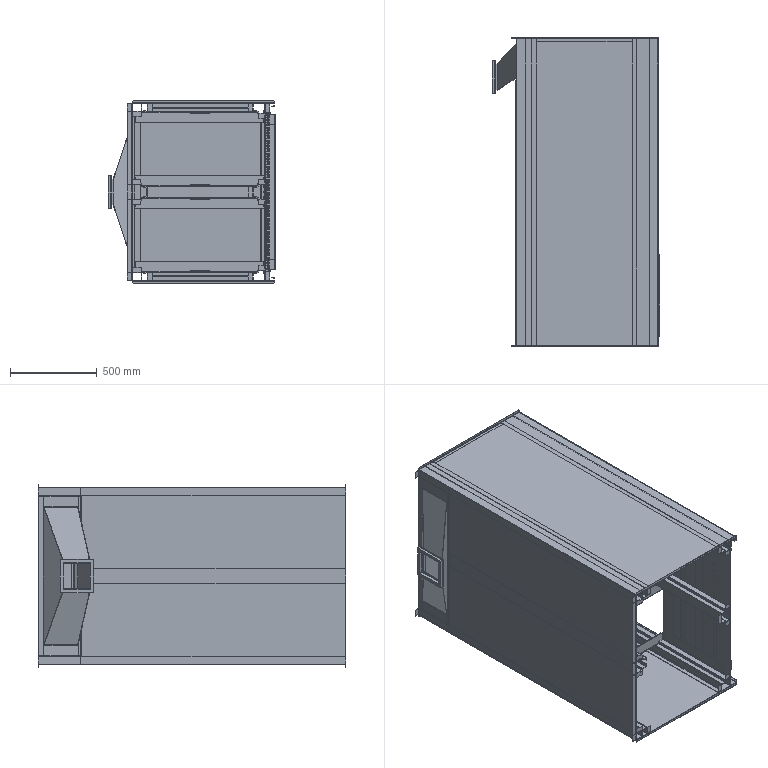Part | SolidWorks | 70 solids | 6901 faces | volume 26326722 mm3 | plane 4145 | cylinder 2728 | spline 28 | commonest cylinder face diameters 8 x968 12 x512 6 x421 7 x240 6.5 x236 2 x86